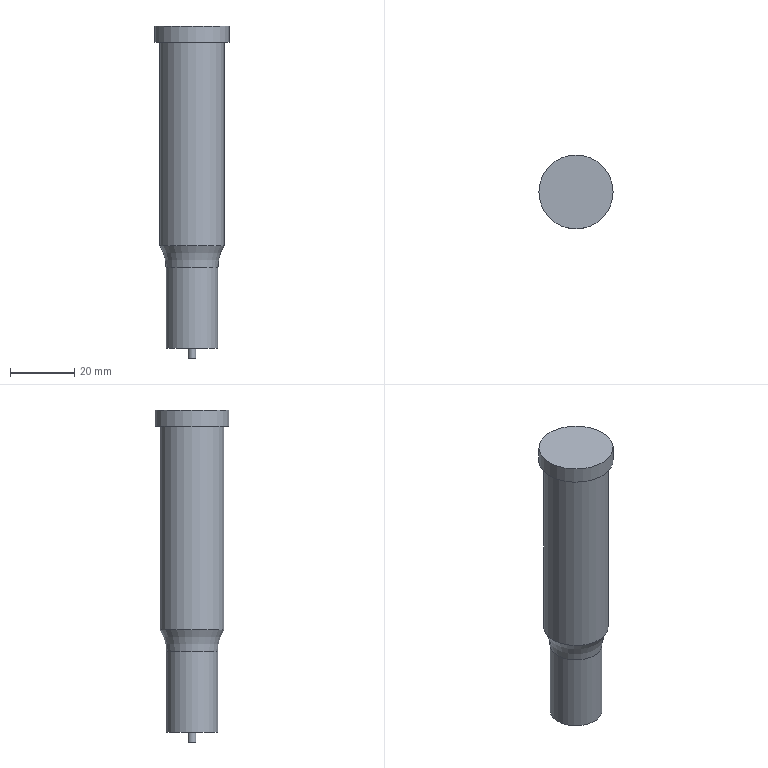Part | STEP file | lll_id3182_x_t | 1 solid | 9 faces | box 23 x 23 x 103 mm | volume 28648 mm3 | cylinder 4 | plane 4 | torus 1 | commonest cylinder face diameters 2.4 x1 16.1 x1 20 x1 23 x1
STEP:
#1=CARTESIAN_POINT('',(427.,-300.,87.5));
#2=VERTEX_POINT('',#1);
#3=CARTESIAN_POINT('',(437.,-300.,87.5));
#4=DIRECTION('',(0.,0.,1.));
#5=DIRECTION('',(-1.,0.,0.));
#6=AXIS2_PLACEMENT_3D('',#3,#4,#5);
#7=CIRCLE('',#6,10.);
#8=EDGE_CURVE('',#2,#2,#7,.T.);
#9=ORIENTED_EDGE('',*,*,#8,.F.);
#10=EDGE_LOOP('',(#9));
#11=FACE_BOUND('',#10,.T.);
#12=CARTESIAN_POINT('',(447.,-300.,24.348));
#13=VERTEX_POINT('',#12);
#14=CARTESIAN_POINT('',(437.,-300.,24.348));
#15=DIRECTION('',(0.,0.,-1.));
#16=DIRECTION('',(1.,0.,0.));
#17=AXIS2_PLACEMENT_3D('',#14,#15,#16);
#18=CIRCLE('',#17,10.);
#19=EDGE_CURVE('',#13,#13,#18,.T.);
#20=ORIENTED_EDGE('',*,*,#19,.F.);
#21=EDGE_LOOP('',(#20));
#22=FACE_BOUND('',#21,.T.);
#23=CARTESIAN_POINT('',(437.,-300.,125.));
#24=DIRECTION('',(0.,0.,-1.));
#25=DIRECTION('',(1.,0.,0.));
#26=AXIS2_PLACEMENT_3D('',#23,#24,#25);
#27=CYLINDRICAL_SURFACE('',#26,10.);
#28=ADVANCED_FACE('',(#11,#22),#27,.T.);
#29=CARTESIAN_POINT('',(425.5,-300.,87.5));
#30=VERTEX_POINT('',#29);
#31=CARTESIAN_POINT('',(437.,-300.,87.5));
#32=DIRECTION('',(0.,0.,-1.));
#33=DIRECTION('',(-1.,0.,0.));
#34=AXIS2_PLACEMENT_3D('',#31,#32,#33);
#35=CIRCLE('',#34,11.5);
#36=EDGE_CURVE('',#30,#30,#35,.T.);
#37=ORIENTED_EDGE('',*,*,#36,.T.);
#38=EDGE_LOOP('',(#37));
#39=FACE_BOUND('',#38,.T.);
#40=ORIENTED_EDGE('',*,*,#8,.T.);
#41=EDGE_LOOP('',(#40));
#42=FACE_BOUND('',#41,.T.);
#43=CARTESIAN_POINT('',(437.,-300.,87.5));
#44=DIRECTION('',(0.,0.,1.));
#45=DIRECTION('',(-1.,0.,0.));
#46=AXIS2_PLACEMENT_3D('',#43,#44,#45);
#47=PLANE('',#46);
#48=ADVANCED_FACE('',(#39,#42),#47,.F.);
#49=CARTESIAN_POINT('',(448.5,-300.,92.5));
#50=VERTEX_POINT('',#49);
#51=CARTESIAN_POINT('',(437.,-300.,92.5));
#52=DIRECTION('',(0.,0.,1.));
#53=DIRECTION('',(1.,0.,0.));
#54=AXIS2_PLACEMENT_3D('',#51,#52,#53);
#55=CIRCLE('',#54,11.5);
#56=EDGE_CURVE('',#50,#50,#55,.T.);
#57=ORIENTED_EDGE('',*,*,#56,.T.);
#58=EDGE_LOOP('',(#57));
#59=FACE_OUTER_BOUND('',#58,.T.);
#60=CARTESIAN_POINT('',(444.,-579.,92.5));
#61=DIRECTION('',(0.,0.,-1.));
#62=DIRECTION('',(1.,0.,0.));
#63=AXIS2_PLACEMENT_3D('',#60,#61,#62);
#64=PLANE('',#63);
#65=ADVANCED_FACE('',(#59),#64,.F.);
#66=ORIENTED_EDGE('',*,*,#36,.F.);
#67=EDGE_LOOP('',(#66));
#68=FACE_BOUND('',#67,.T.);
#69=ORIENTED_EDGE('',*,*,#56,.F.);
#70=EDGE_LOOP('',(#69));
#71=FACE_BOUND('',#70,.T.);
#72=CARTESIAN_POINT('',(437.,-300.,125.));
#73=DIRECTION('',(0.,0.,-1.));
#74=DIRECTION('',(1.,0.,0.));
#75=AXIS2_PLACEMENT_3D('',#72,#73,#74);
#76=CYLINDRICAL_SURFACE('',#75,11.5);
#77=ADVANCED_FACE('',(#68,#71),#76,.T.);
#78=CARTESIAN_POINT('',(435.8,-300.,-10.5));
#79=VERTEX_POINT('',#78);
#80=CARTESIAN_POINT('',(437.,-300.,-10.5));
#81=DIRECTION('',(0.,0.,1.));
#82=DIRECTION('',(-1.,0.,0.));
#83=AXIS2_PLACEMENT_3D('',#80,#81,#82);
#84=CIRCLE('',#83,1.2);
#85=EDGE_CURVE('',#79,#79,#84,.T.);
#86=ORIENTED_EDGE('',*,*,#85,.F.);
#87=EDGE_LOOP('',(#86));
#88=FACE_OUTER_BOUND('',#87,.T.);
#89=CARTESIAN_POINT('',(437.,-300.,-10.5));
#90=DIRECTION('',(0.,0.,-1.));
#91=DIRECTION('',(1.,0.,0.));
#92=AXIS2_PLACEMENT_3D('',#89,#90,#91);
#93=PLANE('',#92);
#94=ADVANCED_FACE('',(#88),#93,.T.);
#95=ORIENTED_EDGE('',*,*,#85,.T.);
#96=EDGE_LOOP('',(#95));
#97=FACE_BOUND('',#96,.T.);
#98=CARTESIAN_POINT('',(435.8,-300.,-7.5));
#99=VERTEX_POINT('',#98);
#100=CARTESIAN_POINT('',(437.,-300.,-7.5));
#101=DIRECTION('',(0.,0.,-1.));
#102=DIRECTION('',(-1.,0.,0.));
#103=AXIS2_PLACEMENT_3D('',#100,#101,#102);
#104=CIRCLE('',#103,1.2);
#105=EDGE_CURVE('',#99,#99,#104,.T.);
#106=ORIENTED_EDGE('',*,*,#105,.T.);
#107=EDGE_LOOP('',(#106));
#108=FACE_BOUND('',#107,.T.);
#109=CARTESIAN_POINT('',(437.,-300.,-7.5));
#110=DIRECTION('',(0.,0.,-1.));
#111=DIRECTION('',(-1.,0.,0.));
#112=AXIS2_PLACEMENT_3D('',#109,#110,#111);
#113=CYLINDRICAL_SURFACE('',#112,1.2);
#114=ADVANCED_FACE('',(#97,#108),#113,.T.);
#115=CARTESIAN_POINT('',(428.95,-300.,-7.5));
#116=VERTEX_POINT('',#115);
#117=CARTESIAN_POINT('',(437.,-300.,-7.5));
#118=DIRECTION('',(0.,0.,1.));
#119=DIRECTION('',(-1.,0.,0.));
#120=AXIS2_PLACEMENT_3D('',#117,#118,#119);
#121=CIRCLE('',#120,8.05);
#122=EDGE_CURVE('',#116,#116,#121,.T.);
#123=ORIENTED_EDGE('',*,*,#122,.F.);
#124=EDGE_LOOP('',(#123));
#125=FACE_BOUND('',#124,.T.);
#126=ORIENTED_EDGE('',*,*,#105,.F.);
#127=EDGE_LOOP('',(#126));
#128=FACE_BOUND('',#127,.T.);
#129=CARTESIAN_POINT('',(437.,-300.,-7.5));
#130=DIRECTION('',(0.,0.,1.));
#131=DIRECTION('',(-1.,0.,0.));
#132=AXIS2_PLACEMENT_3D('',#129,#130,#131);
#133=PLANE('',#132);
#134=ADVANCED_FACE('',(#125,#128),#133,.F.);
#135=CARTESIAN_POINT('',(428.95,-300.,17.5));
#136=VERTEX_POINT('',#135);
#137=CARTESIAN_POINT('',(437.,-300.,17.5));
#138=DIRECTION('',(0.,0.,-1.));
#139=DIRECTION('',(-1.,0.,0.));
#140=AXIS2_PLACEMENT_3D('',#137,#138,#139);
#141=CIRCLE('',#140,8.05);
#142=EDGE_CURVE('',#136,#136,#141,.T.);
#143=ORIENTED_EDGE('',*,*,#142,.T.);
#144=EDGE_LOOP('',(#143));
#145=FACE_BOUND('',#144,.T.);
#146=ORIENTED_EDGE('',*,*,#122,.T.);
#147=EDGE_LOOP('',(#146));
#148=FACE_BOUND('',#147,.T.);
#149=CARTESIAN_POINT('',(437.,-300.,125.));
#150=DIRECTION('',(0.,0.,-1.));
#151=DIRECTION('',(1.,0.,0.));
#152=AXIS2_PLACEMENT_3D('',#149,#150,#151);
#153=CYLINDRICAL_SURFACE('',#152,8.05);
#154=ADVANCED_FACE('',(#145,#148),#153,.T.);
#155=ORIENTED_EDGE('',*,*,#19,.T.);
#156=EDGE_LOOP('',(#155));
#157=FACE_BOUND('',#156,.T.);
#158=ORIENTED_EDGE('',*,*,#142,.F.);
#159=EDGE_LOOP('',(#158));
#160=FACE_BOUND('',#159,.T.);
#161=CARTESIAN_POINT('',(437.,-300.,17.5));
#162=DIRECTION('',(0.,0.,1.));
#163=DIRECTION('',(-1.,0.,0.));
#164=AXIS2_PLACEMENT_3D('',#161,#162,#163);
#165=TOROIDAL_SURFACE('',#164,21.05,13.);
#166=ADVANCED_FACE('',(#157,#160),#165,.F.);
#167=CLOSED_SHELL('',(#28,#48,#65,#77,#94,#114,#134,#154,#166));
#168=MANIFOLD_SOLID_BREP('',#167);
#169=(LENGTH_UNIT()NAMED_UNIT(*)SI_UNIT(.MILLI.,.METRE.));
#170=UNCERTAINTY_MEASURE_WITH_UNIT(LENGTH_MEASURE(0.00002),#169,'','');
#171=(NAMED_UNIT(*)PLANE_ANGLE_UNIT()SI_UNIT($,.RADIAN.));
#172=PLANE_ANGLE_MEASURE_WITH_UNIT(PLANE_ANGLE_MEASURE(0.01745),#171);
#173=DIMENSIONAL_EXPONENTS(0.,0.,0.,0.,0.,0.,0.);
#174=(CONVERSION_BASED_UNIT('DEGREE',#172)NAMED_UNIT(#173)PLANE_ANGLE_UNIT());
#175=(NAMED_UNIT(*)SI_UNIT($,.STERADIAN.)SOLID_ANGLE_UNIT());
#176=(GEOMETRIC_REPRESENTATION_CONTEXT(3)GLOBAL_UNCERTAINTY_ASSIGNED_CONTEXT((#170))GLOBAL_UNIT_ASSIGNED_CONTEXT((#169,#174,#175))REPRESENTATION_CONTEXT('',''));
#177=ADVANCED_BREP_SHAPE_REPRESENTATION('',(#168),#176);